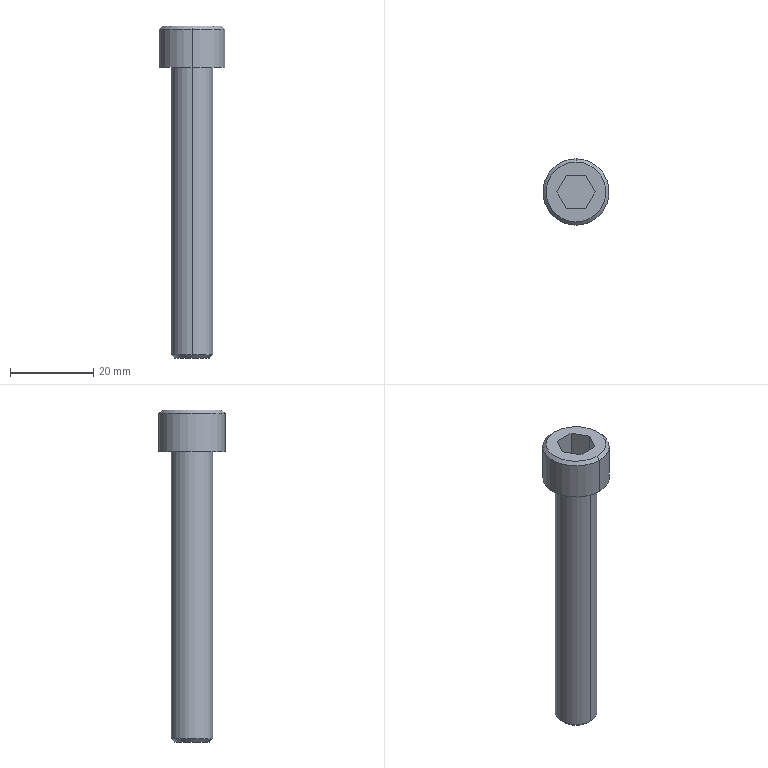Part | Creo | 1 solid | 18 faces | box 16 x 16 x 80 mm | volume 7152 mm3 | plane 10 | cylinder 4 | cone 4 | commonest cylinder face diameters 10 x2 16 x2
STEP:
#1=CARTESIAN_POINT('',(130.5,269.,-13.5));
#2=VERTEX_POINT('',#1);
#3=CARTESIAN_POINT('',(130.5,285.,-13.5));
#4=VERTEX_POINT('',#3);
#5=CARTESIAN_POINT('',(130.5,277.,-13.5));
#6=DIRECTION('',(0.,0.,-1.));
#7=DIRECTION('',(0.,-1.,0.));
#8=AXIS2_PLACEMENT_3D('',#5,#6,#7);
#9=CIRCLE('',#8,8.);
#10=EDGE_CURVE('',#2,#4,#9,.T.);
#11=ORIENTED_EDGE('',*,*,#10,.F.);
#12=CARTESIAN_POINT('',(130.5,277.,-13.5));
#13=DIRECTION('',(0.,0.,-1.));
#14=DIRECTION('',(0.,1.,0.));
#15=AXIS2_PLACEMENT_3D('',#12,#13,#14);
#16=CIRCLE('',#15,8.);
#17=EDGE_CURVE('',#4,#2,#16,.T.);
#18=ORIENTED_EDGE('',*,*,#17,.F.);
#19=EDGE_LOOP('',(#11,#18));
#20=FACE_OUTER_BOUND('',#19,.F.);
#21=CARTESIAN_POINT('',(130.5,282.,-13.5));
#22=VERTEX_POINT('',#21);
#23=CARTESIAN_POINT('',(130.5,272.,-13.5));
#24=VERTEX_POINT('',#23);
#25=CARTESIAN_POINT('',(130.5,277.,-13.5));
#26=DIRECTION('',(0.,0.,1.));
#27=DIRECTION('',(0.,1.,0.));
#28=AXIS2_PLACEMENT_3D('',#25,#26,#27);
#29=CIRCLE('',#28,5.);
#30=EDGE_CURVE('',#22,#24,#29,.T.);
#31=ORIENTED_EDGE('',*,*,#30,.F.);
#32=CARTESIAN_POINT('',(130.5,277.,-13.5));
#33=DIRECTION('',(0.,0.,1.));
#34=DIRECTION('',(0.,-1.,0.));
#35=AXIS2_PLACEMENT_3D('',#32,#33,#34);
#36=CIRCLE('',#35,5.);
#37=EDGE_CURVE('',#24,#22,#36,.T.);
#38=ORIENTED_EDGE('',*,*,#37,.F.);
#39=EDGE_LOOP('',(#31,#38));
#40=FACE_BOUND('',#39,.F.);
#41=CARTESIAN_POINT('',(130.5,277.,-13.5));
#42=DIRECTION('',(0.,0.,-1.));
#43=DIRECTION('',(0.,1.,0.));
#44=AXIS2_PLACEMENT_3D('',#41,#42,#43);
#45=PLANE('',#44);
#46=ADVANCED_FACE('',(#20,#40),#45,.T.);
#47=CARTESIAN_POINT('',(130.5,272.,-82.75));
#48=VERTEX_POINT('',#47);
#49=CARTESIAN_POINT('',(130.5,282.,-82.75));
#50=VERTEX_POINT('',#49);
#51=CARTESIAN_POINT('',(130.5,277.,-82.75));
#52=DIRECTION('',(0.,0.,-1.));
#53=DIRECTION('',(0.,-1.,0.));
#54=AXIS2_PLACEMENT_3D('',#51,#52,#53);
#55=CIRCLE('',#54,5.);
#56=EDGE_CURVE('',#48,#50,#55,.T.);
#57=ORIENTED_EDGE('',*,*,#56,.T.);
#58=CARTESIAN_POINT('',(130.5,282.,-13.5));
#59=DIRECTION('',(0.,0.,-1.));
#60=VECTOR('',#59,69.25);
#61=LINE('',#58,#60);
#62=EDGE_CURVE('',#22,#50,#61,.T.);
#63=ORIENTED_EDGE('',*,*,#62,.F.);
#64=ORIENTED_EDGE('',*,*,#30,.T.);
#65=CARTESIAN_POINT('',(130.5,272.,-13.5));
#66=DIRECTION('',(0.,0.,-1.));
#67=VECTOR('',#66,69.25);
#68=LINE('',#65,#67);
#69=EDGE_CURVE('',#24,#48,#68,.T.);
#70=ORIENTED_EDGE('',*,*,#69,.T.);
#71=EDGE_LOOP('',(#57,#63,#64,#70));
#72=FACE_OUTER_BOUND('',#71,.F.);
#73=CARTESIAN_POINT('',(130.5,277.,-1.5));
#74=DIRECTION('',(0.,0.,-1.));
#75=DIRECTION('',(0.,1.,0.));
#76=AXIS2_PLACEMENT_3D('',#73,#74,#75);
#77=CYLINDRICAL_SURFACE('',#76,5.);
#78=ADVANCED_FACE('',(#72),#77,.T.);
#79=CARTESIAN_POINT('',(130.5,272.75,-83.5));
#80=VERTEX_POINT('',#79);
#81=CARTESIAN_POINT('',(130.5,281.25,-83.5));
#82=VERTEX_POINT('',#81);
#83=CARTESIAN_POINT('',(130.5,277.,-83.5));
#84=DIRECTION('',(0.,0.,-1.));
#85=DIRECTION('',(0.,-1.,0.));
#86=AXIS2_PLACEMENT_3D('',#83,#84,#85);
#87=CIRCLE('',#86,4.25);
#88=EDGE_CURVE('',#80,#82,#87,.T.);
#89=ORIENTED_EDGE('',*,*,#88,.T.);
#90=CARTESIAN_POINT('',(130.5,281.25,-83.5));
#91=DIRECTION('',(0.,0.7071,0.7071));
#92=VECTOR('',#91,1.061);
#93=LINE('',#90,#92);
#94=EDGE_CURVE('',#82,#50,#93,.T.);
#95=ORIENTED_EDGE('',*,*,#94,.T.);
#96=ORIENTED_EDGE('',*,*,#56,.F.);
#97=CARTESIAN_POINT('',(130.5,272.75,-83.5));
#98=DIRECTION('',(0.,-0.7071,0.7071));
#99=VECTOR('',#98,1.061);
#100=LINE('',#97,#99);
#101=EDGE_CURVE('',#80,#48,#100,.T.);
#102=ORIENTED_EDGE('',*,*,#101,.F.);
#103=EDGE_LOOP('',(#89,#95,#96,#102));
#104=FACE_OUTER_BOUND('',#103,.F.);
#105=CARTESIAN_POINT('',(130.5,277.,-83.125));
#106=DIRECTION('',(0.,0.,1.));
#107=DIRECTION('',(0.,-1.,0.));
#108=AXIS2_PLACEMENT_3D('',#105,#106,#107);
#109=CONICAL_SURFACE('',#108,4.625,45.);
#110=ADVANCED_FACE('',(#104),#109,.T.);
#111=CARTESIAN_POINT('',(130.5,277.,-83.5));
#112=DIRECTION('',(0.,0.,-1.));
#113=DIRECTION('',(0.,1.,0.));
#114=AXIS2_PLACEMENT_3D('',#111,#112,#113);
#115=CIRCLE('',#114,4.25);
#116=EDGE_CURVE('',#82,#80,#115,.T.);
#117=ORIENTED_EDGE('',*,*,#116,.F.);
#118=ORIENTED_EDGE('',*,*,#88,.F.);
#119=EDGE_LOOP('',(#117,#118));
#120=FACE_OUTER_BOUND('',#119,.F.);
#121=CARTESIAN_POINT('',(130.5,277.,-83.5));
#122=DIRECTION('',(0.,0.,-1.));
#123=DIRECTION('',(0.,1.,0.));
#124=AXIS2_PLACEMENT_3D('',#121,#122,#123);
#125=PLANE('',#124);
#126=ADVANCED_FACE('',(#120),#125,.T.);
#127=ORIENTED_EDGE('',*,*,#116,.T.);
#128=ORIENTED_EDGE('',*,*,#101,.T.);
#129=CARTESIAN_POINT('',(130.5,277.,-82.75));
#130=DIRECTION('',(0.,0.,-1.));
#131=DIRECTION('',(0.,1.,0.));
#132=AXIS2_PLACEMENT_3D('',#129,#130,#131);
#133=CIRCLE('',#132,5.);
#134=EDGE_CURVE('',#50,#48,#133,.T.);
#135=ORIENTED_EDGE('',*,*,#134,.F.);
#136=ORIENTED_EDGE('',*,*,#94,.F.);
#137=EDGE_LOOP('',(#127,#128,#135,#136));
#138=FACE_OUTER_BOUND('',#137,.F.);
#139=CARTESIAN_POINT('',(130.5,277.,-83.125));
#140=DIRECTION('',(0.,0.,1.));
#141=DIRECTION('',(0.,-1.,0.));
#142=AXIS2_PLACEMENT_3D('',#139,#140,#141);
#143=CONICAL_SURFACE('',#142,4.625,45.);
#144=ADVANCED_FACE('',(#138),#143,.T.);
#145=ORIENTED_EDGE('',*,*,#134,.T.);
#146=ORIENTED_EDGE('',*,*,#69,.F.);
#147=ORIENTED_EDGE('',*,*,#37,.T.);
#148=ORIENTED_EDGE('',*,*,#62,.T.);
#149=EDGE_LOOP('',(#145,#146,#147,#148));
#150=FACE_OUTER_BOUND('',#149,.F.);
#151=CARTESIAN_POINT('',(130.5,277.,-1.5));
#152=DIRECTION('',(0.,0.,-1.));
#153=DIRECTION('',(0.,1.,0.));
#154=AXIS2_PLACEMENT_3D('',#151,#152,#153);
#155=CYLINDRICAL_SURFACE('',#154,5.);
#156=ADVANCED_FACE('',(#150),#155,.T.);
#157=CARTESIAN_POINT('',(130.5,285.,-4.3));
#158=VERTEX_POINT('',#157);
#159=CARTESIAN_POINT('',(130.5,269.,-4.3));
#160=VERTEX_POINT('',#159);
#161=CARTESIAN_POINT('',(130.5,277.,-4.3));
#162=DIRECTION('',(0.,0.,1.));
#163=DIRECTION('',(0.,1.,0.));
#164=AXIS2_PLACEMENT_3D('',#161,#162,#163);
#165=CIRCLE('',#164,8.);
#166=EDGE_CURVE('',#158,#160,#165,.T.);
#167=ORIENTED_EDGE('',*,*,#166,.T.);
#168=CARTESIAN_POINT('',(130.5,269.,-4.3));
#169=DIRECTION('',(0.,0.,-1.));
#170=VECTOR('',#169,9.2);
#171=LINE('',#168,#170);
#172=EDGE_CURVE('',#160,#2,#171,.T.);
#173=ORIENTED_EDGE('',*,*,#172,.T.);
#174=ORIENTED_EDGE('',*,*,#10,.T.);
#175=CARTESIAN_POINT('',(130.5,285.,-4.3));
#176=DIRECTION('',(0.,0.,-1.));
#177=VECTOR('',#176,9.2);
#178=LINE('',#175,#177);
#179=EDGE_CURVE('',#158,#4,#178,.T.);
#180=ORIENTED_EDGE('',*,*,#179,.F.);
#181=EDGE_LOOP('',(#167,#173,#174,#180));
#182=FACE_OUTER_BOUND('',#181,.F.);
#183=CARTESIAN_POINT('',(130.5,277.,-1.5));
#184=DIRECTION('',(0.,0.,-1.));
#185=DIRECTION('',(0.,1.,0.));
#186=AXIS2_PLACEMENT_3D('',#183,#184,#185);
#187=CYLINDRICAL_SURFACE('',#186,8.);
#188=ADVANCED_FACE('',(#182),#187,.T.);
#189=CARTESIAN_POINT('',(130.5,284.2,-3.5));
#190=VERTEX_POINT('',#189);
#191=CARTESIAN_POINT('',(130.5,269.8,-3.5));
#192=VERTEX_POINT('',#191);
#193=CARTESIAN_POINT('',(130.5,277.,-3.5));
#194=DIRECTION('',(0.,0.,1.));
#195=DIRECTION('',(0.,1.,0.));
#196=AXIS2_PLACEMENT_3D('',#193,#194,#195);
#197=CIRCLE('',#196,7.2);
#198=EDGE_CURVE('',#190,#192,#197,.T.);
#199=ORIENTED_EDGE('',*,*,#198,.T.);
#200=CARTESIAN_POINT('',(130.5,269.8,-3.5));
#201=DIRECTION('',(0.,-0.7071,-0.7071));
#202=VECTOR('',#201,1.131);
#203=LINE('',#200,#202);
#204=EDGE_CURVE('',#192,#160,#203,.T.);
#205=ORIENTED_EDGE('',*,*,#204,.T.);
#206=ORIENTED_EDGE('',*,*,#166,.F.);
#207=CARTESIAN_POINT('',(130.5,284.2,-3.5));
#208=DIRECTION('',(0.,0.7071,-0.7071));
#209=VECTOR('',#208,1.131);
#210=LINE('',#207,#209);
#211=EDGE_CURVE('',#190,#158,#210,.T.);
#212=ORIENTED_EDGE('',*,*,#211,.F.);
#213=EDGE_LOOP('',(#199,#205,#206,#212));
#214=FACE_OUTER_BOUND('',#213,.F.);
#215=CARTESIAN_POINT('',(130.5,277.,-3.9));
#216=DIRECTION('',(0.,0.,-1.));
#217=DIRECTION('',(0.,1.,0.));
#218=AXIS2_PLACEMENT_3D('',#215,#216,#217);
#219=CONICAL_SURFACE('',#218,7.6,45.);
#220=ADVANCED_FACE('',(#214),#219,.T.);
#221=ORIENTED_EDGE('',*,*,#198,.F.);
#222=CARTESIAN_POINT('',(130.5,277.,-3.5));
#223=DIRECTION('',(0.,0.,1.));
#224=DIRECTION('',(0.,-1.,0.));
#225=AXIS2_PLACEMENT_3D('',#222,#223,#224);
#226=CIRCLE('',#225,7.2);
#227=EDGE_CURVE('',#192,#190,#226,.T.);
#228=ORIENTED_EDGE('',*,*,#227,.F.);
#229=EDGE_LOOP('',(#221,#228));
#230=FACE_OUTER_BOUND('',#229,.F.);
#231=CARTESIAN_POINT('',(128.191,273.,-3.5));
#232=VERTEX_POINT('',#231);
#233=CARTESIAN_POINT('',(125.881,277.,-3.5));
#234=VERTEX_POINT('',#233);
#235=CARTESIAN_POINT('',(128.191,273.,-3.5));
#236=DIRECTION('',(-0.5,0.866,0.));
#237=VECTOR('',#236,4.619);
#238=LINE('',#235,#237);
#239=EDGE_CURVE('',#232,#234,#238,.T.);
#240=ORIENTED_EDGE('',*,*,#239,.F.);
#241=CARTESIAN_POINT('',(132.809,273.,-3.5));
#242=VERTEX_POINT('',#241);
#243=CARTESIAN_POINT('',(132.809,273.,-3.5));
#244=DIRECTION('',(-1.,0.,0.));
#245=VECTOR('',#244,4.619);
#246=LINE('',#243,#245);
#247=EDGE_CURVE('',#242,#232,#246,.T.);
#248=ORIENTED_EDGE('',*,*,#247,.F.);
#249=CARTESIAN_POINT('',(135.119,277.,-3.5));
#250=VERTEX_POINT('',#249);
#251=CARTESIAN_POINT('',(135.119,277.,-3.5));
#252=DIRECTION('',(-0.5,-0.866,0.));
#253=VECTOR('',#252,4.619);
#254=LINE('',#251,#253);
#255=EDGE_CURVE('',#250,#242,#254,.T.);
#256=ORIENTED_EDGE('',*,*,#255,.F.);
#257=CARTESIAN_POINT('',(132.809,281.,-3.5));
#258=VERTEX_POINT('',#257);
#259=CARTESIAN_POINT('',(132.809,281.,-3.5));
#260=DIRECTION('',(0.5,-0.866,0.));
#261=VECTOR('',#260,4.619);
#262=LINE('',#259,#261);
#263=EDGE_CURVE('',#258,#250,#262,.T.);
#264=ORIENTED_EDGE('',*,*,#263,.F.);
#265=CARTESIAN_POINT('',(128.191,281.,-3.5));
#266=VERTEX_POINT('',#265);
#267=CARTESIAN_POINT('',(128.191,281.,-3.5));
#268=DIRECTION('',(1.,0.,0.));
#269=VECTOR('',#268,4.619);
#270=LINE('',#267,#269);
#271=EDGE_CURVE('',#266,#258,#270,.T.);
#272=ORIENTED_EDGE('',*,*,#271,.F.);
#273=CARTESIAN_POINT('',(125.881,277.,-3.5));
#274=DIRECTION('',(0.5,0.866,0.));
#275=VECTOR('',#274,4.619);
#276=LINE('',#273,#275);
#277=EDGE_CURVE('',#234,#266,#276,.T.);
#278=ORIENTED_EDGE('',*,*,#277,.F.);
#279=EDGE_LOOP('',(#240,#248,#256,#264,#272,#278));
#280=FACE_BOUND('',#279,.F.);
#281=CARTESIAN_POINT('',(130.5,277.,-3.5));
#282=DIRECTION('',(0.,0.,-1.));
#283=DIRECTION('',(0.,1.,0.));
#284=AXIS2_PLACEMENT_3D('',#281,#282,#283);
#285=PLANE('',#284);
#286=ADVANCED_FACE('',(#230,#280),#285,.F.);
#287=ORIENTED_EDGE('',*,*,#227,.T.);
#288=ORIENTED_EDGE('',*,*,#211,.T.);
#289=CARTESIAN_POINT('',(130.5,277.,-4.3));
#290=DIRECTION('',(0.,0.,1.));
#291=DIRECTION('',(0.,-1.,0.));
#292=AXIS2_PLACEMENT_3D('',#289,#290,#291);
#293=CIRCLE('',#292,8.);
#294=EDGE_CURVE('',#160,#158,#293,.T.);
#295=ORIENTED_EDGE('',*,*,#294,.F.);
#296=ORIENTED_EDGE('',*,*,#204,.F.);
#297=EDGE_LOOP('',(#287,#288,#295,#296));
#298=FACE_OUTER_BOUND('',#297,.F.);
#299=CARTESIAN_POINT('',(130.5,277.,-3.9));
#300=DIRECTION('',(0.,0.,-1.));
#301=DIRECTION('',(0.,1.,0.));
#302=AXIS2_PLACEMENT_3D('',#299,#300,#301);
#303=CONICAL_SURFACE('',#302,7.6,45.);
#304=ADVANCED_FACE('',(#298),#303,.T.);
#305=ORIENTED_EDGE('',*,*,#294,.T.);
#306=ORIENTED_EDGE('',*,*,#179,.T.);
#307=ORIENTED_EDGE('',*,*,#17,.T.);
#308=ORIENTED_EDGE('',*,*,#172,.F.);
#309=EDGE_LOOP('',(#305,#306,#307,#308));
#310=FACE_OUTER_BOUND('',#309,.F.);
#311=CARTESIAN_POINT('',(130.5,277.,-1.5));
#312=DIRECTION('',(0.,0.,-1.));
#313=DIRECTION('',(0.,1.,0.));
#314=AXIS2_PLACEMENT_3D('',#311,#312,#313);
#315=CYLINDRICAL_SURFACE('',#314,8.);
#316=ADVANCED_FACE('',(#310),#315,.T.);
#317=ORIENTED_EDGE('',*,*,#239,.T.);
#318=CARTESIAN_POINT('',(125.881,277.,-9.5));
#319=VERTEX_POINT('',#318);
#320=CARTESIAN_POINT('',(125.881,277.,-3.5));
#321=DIRECTION('',(0.,0.,-1.));
#322=VECTOR('',#321,6.);
#323=LINE('',#320,#322);
#324=EDGE_CURVE('',#234,#319,#323,.T.);
#325=ORIENTED_EDGE('',*,*,#324,.T.);
#326=CARTESIAN_POINT('',(128.191,273.,-9.5));
#327=VERTEX_POINT('',#326);
#328=CARTESIAN_POINT('',(125.881,277.,-9.5));
#329=DIRECTION('',(0.5,-0.866,0.));
#330=VECTOR('',#329,4.619);
#331=LINE('',#328,#330);
#332=EDGE_CURVE('',#319,#327,#331,.T.);
#333=ORIENTED_EDGE('',*,*,#332,.T.);
#334=CARTESIAN_POINT('',(128.191,273.,-3.5));
#335=DIRECTION('',(0.,0.,-1.));
#336=VECTOR('',#335,6.);
#337=LINE('',#334,#336);
#338=EDGE_CURVE('',#232,#327,#337,.T.);
#339=ORIENTED_EDGE('',*,*,#338,.F.);
#340=EDGE_LOOP('',(#317,#325,#333,#339));
#341=FACE_OUTER_BOUND('',#340,.F.);
#342=CARTESIAN_POINT('',(125.881,277.,-9.5));
#343=DIRECTION('',(-0.866,-0.5,0.));
#344=DIRECTION('',(0.5,-0.866,0.));
#345=AXIS2_PLACEMENT_3D('',#342,#343,#344);
#346=PLANE('',#345);
#347=ADVANCED_FACE('',(#341),#346,.F.);
#348=ORIENTED_EDGE('',*,*,#277,.T.);
#349=CARTESIAN_POINT('',(128.191,281.,-9.5));
#350=VERTEX_POINT('',#349);
#351=CARTESIAN_POINT('',(128.191,281.,-3.5));
#352=DIRECTION('',(0.,0.,-1.));
#353=VECTOR('',#352,6.);
#354=LINE('',#351,#353);
#355=EDGE_CURVE('',#266,#350,#354,.T.);
#356=ORIENTED_EDGE('',*,*,#355,.T.);
#357=CARTESIAN_POINT('',(128.191,281.,-9.5));
#358=DIRECTION('',(-0.5,-0.866,0.));
#359=VECTOR('',#358,4.619);
#360=LINE('',#357,#359);
#361=EDGE_CURVE('',#350,#319,#360,.T.);
#362=ORIENTED_EDGE('',*,*,#361,.T.);
#363=ORIENTED_EDGE('',*,*,#324,.F.);
#364=EDGE_LOOP('',(#348,#356,#362,#363));
#365=FACE_OUTER_BOUND('',#364,.F.);
#366=CARTESIAN_POINT('',(128.191,281.,-9.5));
#367=DIRECTION('',(-0.866,0.5,0.));
#368=DIRECTION('',(-0.5,-0.866,0.));
#369=AXIS2_PLACEMENT_3D('',#366,#367,#368);
#370=PLANE('',#369);
#371=ADVANCED_FACE('',(#365),#370,.F.);
#372=ORIENTED_EDGE('',*,*,#271,.T.);
#373=CARTESIAN_POINT('',(132.809,281.,-9.5));
#374=VERTEX_POINT('',#373);
#375=CARTESIAN_POINT('',(132.809,281.,-3.5));
#376=DIRECTION('',(0.,0.,-1.));
#377=VECTOR('',#376,6.);
#378=LINE('',#375,#377);
#379=EDGE_CURVE('',#258,#374,#378,.T.);
#380=ORIENTED_EDGE('',*,*,#379,.T.);
#381=CARTESIAN_POINT('',(128.191,281.,-9.5));
#382=DIRECTION('',(1.,0.,0.));
#383=VECTOR('',#382,4.619);
#384=LINE('',#381,#383);
#385=EDGE_CURVE('',#350,#374,#384,.T.);
#386=ORIENTED_EDGE('',*,*,#385,.F.);
#387=ORIENTED_EDGE('',*,*,#355,.F.);
#388=EDGE_LOOP('',(#372,#380,#386,#387));
#389=FACE_OUTER_BOUND('',#388,.F.);
#390=CARTESIAN_POINT('',(132.809,281.,-9.5));
#391=DIRECTION('',(0.,1.,0.));
#392=DIRECTION('',(0.,0.,1.));
#393=AXIS2_PLACEMENT_3D('',#390,#391,#392);
#394=PLANE('',#393);
#395=ADVANCED_FACE('',(#389),#394,.F.);
#396=ORIENTED_EDGE('',*,*,#263,.T.);
#397=CARTESIAN_POINT('',(135.119,277.,-9.5));
#398=VERTEX_POINT('',#397);
#399=CARTESIAN_POINT('',(135.119,277.,-3.5));
#400=DIRECTION('',(0.,0.,-1.));
#401=VECTOR('',#400,6.);
#402=LINE('',#399,#401);
#403=EDGE_CURVE('',#250,#398,#402,.T.);
#404=ORIENTED_EDGE('',*,*,#403,.T.);
#405=CARTESIAN_POINT('',(135.119,277.,-9.5));
#406=DIRECTION('',(-0.5,0.866,0.));
#407=VECTOR('',#406,4.619);
#408=LINE('',#405,#407);
#409=EDGE_CURVE('',#398,#374,#408,.T.);
#410=ORIENTED_EDGE('',*,*,#409,.T.);
#411=ORIENTED_EDGE('',*,*,#379,.F.);
#412=EDGE_LOOP('',(#396,#404,#410,#411));
#413=FACE_OUTER_BOUND('',#412,.F.);
#414=CARTESIAN_POINT('',(135.119,277.,-9.5));
#415=DIRECTION('',(0.866,0.5,0.));
#416=DIRECTION('',(-0.5,0.866,0.));
#417=AXIS2_PLACEMENT_3D('',#414,#415,#416);
#418=PLANE('',#417);
#419=ADVANCED_FACE('',(#413),#418,.F.);
#420=ORIENTED_EDGE('',*,*,#255,.T.);
#421=CARTESIAN_POINT('',(132.809,273.,-9.5));
#422=VERTEX_POINT('',#421);
#423=CARTESIAN_POINT('',(132.809,273.,-3.5));
#424=DIRECTION('',(0.,0.,-1.));
#425=VECTOR('',#424,6.);
#426=LINE('',#423,#425);
#427=EDGE_CURVE('',#242,#422,#426,.T.);
#428=ORIENTED_EDGE('',*,*,#427,.T.);
#429=CARTESIAN_POINT('',(132.809,273.,-9.5));
#430=DIRECTION('',(0.5,0.866,0.));
#431=VECTOR('',#430,4.619);
#432=LINE('',#429,#431);
#433=EDGE_CURVE('',#422,#398,#432,.T.);
#434=ORIENTED_EDGE('',*,*,#433,.T.);
#435=ORIENTED_EDGE('',*,*,#403,.F.);
#436=EDGE_LOOP('',(#420,#428,#434,#435));
#437=FACE_OUTER_BOUND('',#436,.F.);
#438=CARTESIAN_POINT('',(132.809,273.,-9.5));
#439=DIRECTION('',(0.866,-0.5,0.));
#440=DIRECTION('',(0.5,0.866,0.));
#441=AXIS2_PLACEMENT_3D('',#438,#439,#440);
#442=PLANE('',#441);
#443=ADVANCED_FACE('',(#437),#442,.F.);
#444=ORIENTED_EDGE('',*,*,#247,.T.);
#445=ORIENTED_EDGE('',*,*,#338,.T.);
#446=CARTESIAN_POINT('',(132.809,273.,-9.5));
#447=DIRECTION('',(-1.,0.,0.));
#448=VECTOR('',#447,4.619);
#449=LINE('',#446,#448);
#450=EDGE_CURVE('',#422,#327,#449,.T.);
#451=ORIENTED_EDGE('',*,*,#450,.F.);
#452=ORIENTED_EDGE('',*,*,#427,.F.);
#453=EDGE_LOOP('',(#444,#445,#451,#452));
#454=FACE_OUTER_BOUND('',#453,.F.);
#455=CARTESIAN_POINT('',(128.191,273.,-9.5));
#456=DIRECTION('',(0.,-1.,0.));
#457=DIRECTION('',(0.,0.,-1.));
#458=AXIS2_PLACEMENT_3D('',#455,#456,#457);
#459=PLANE('',#458);
#460=ADVANCED_FACE('',(#454),#459,.F.);
#461=ORIENTED_EDGE('',*,*,#361,.F.);
#462=ORIENTED_EDGE('',*,*,#385,.T.);
#463=ORIENTED_EDGE('',*,*,#409,.F.);
#464=ORIENTED_EDGE('',*,*,#433,.F.);
#465=ORIENTED_EDGE('',*,*,#450,.T.);
#466=ORIENTED_EDGE('',*,*,#332,.F.);
#467=EDGE_LOOP('',(#461,#462,#463,#464,#465,#466));
#468=FACE_OUTER_BOUND('',#467,.F.);
#469=CARTESIAN_POINT('',(123.572,273.,-9.5));
#470=DIRECTION('',(0.,0.,1.));
#471=DIRECTION('',(0.,-1.,0.));
#472=AXIS2_PLACEMENT_3D('',#469,#470,#471);
#473=PLANE('',#472);
#474=ADVANCED_FACE('',(#468),#473,.T.);
#475=CLOSED_SHELL('',(#46,#78,#110,#126,#144,#156,#188,#220,#286,#304,#316,#347,#371,#395,#419,#443,#460,#474));
#476=MANIFOLD_SOLID_BREP('',#475);
#477=(LENGTH_UNIT()NAMED_UNIT(*)SI_UNIT(.MILLI.,.METRE.));
#478=UNCERTAINTY_MEASURE_WITH_UNIT(LENGTH_MEASURE(0.008314),#477,'','');
#479=(NAMED_UNIT(*)PLANE_ANGLE_UNIT()SI_UNIT($,.RADIAN.));
#480=PLANE_ANGLE_MEASURE_WITH_UNIT(PLANE_ANGLE_MEASURE(0.01745),#479);
#481=(CONVERSION_BASED_UNIT('DEGREE',#480)NAMED_UNIT(*)PLANE_ANGLE_UNIT());
#482=(NAMED_UNIT(*)SI_UNIT($,.STERADIAN.)SOLID_ANGLE_UNIT());
#483=(GEOMETRIC_REPRESENTATION_CONTEXT(3)GLOBAL_UNCERTAINTY_ASSIGNED_CONTEXT((#478))GLOBAL_UNIT_ASSIGNED_CONTEXT((#477,#481,#482))REPRESENTATION_CONTEXT('',''));
#484=ADVANCED_BREP_SHAPE_REPRESENTATION('',(#476),#483);